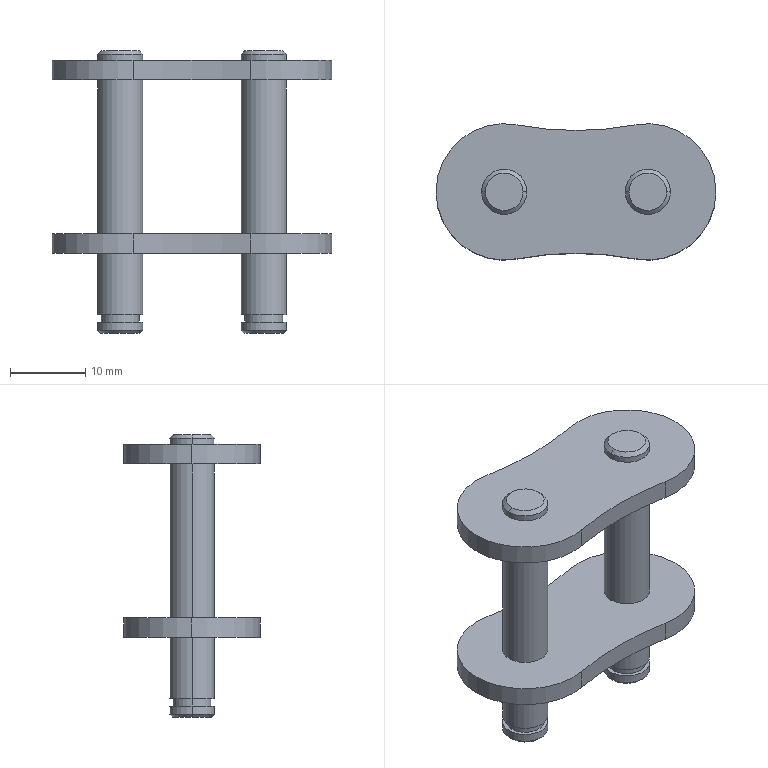Part | SolidWorks | features BaseBody 1 | 1 solid | 50 faces | box 37.13 x 18.08 x 37.5 mm | volume 4809 mm3 | cylinder 30 | plane 12 | cone 8 | commonest cylinder face diameters 6 x16 18.08 x6 5 x4 83.18 x4
STEP:
#1=CARTESIAN_POINT('',(-7.824,-8.879,2.59));
#2=VERTEX_POINT('',#1);
#3=CARTESIAN_POINT('',(-18.565,0.,2.59));
#4=VERTEX_POINT('',#3);
#5=CARTESIAN_POINT('',(-9.525,0.,2.59));
#6=DIRECTION('',(0.,0.,-1.));
#7=DIRECTION('',(-1.,0.,0.));
#8=AXIS2_PLACEMENT_3D('',#5,#6,#7);
#9=CIRCLE('',#8,9.04);
#10=EDGE_CURVE('',#2,#4,#9,.T.);
#11=ORIENTED_EDGE('',*,*,#10,.T.);
#12=CARTESIAN_POINT('',(-18.565,0.,0.));
#13=VERTEX_POINT('',#12);
#14=CARTESIAN_POINT('',(-18.565,0.,2.59));
#15=DIRECTION('',(0.,0.,-1.));
#16=VECTOR('',#15,1000.);
#17=LINE('',#14,#16);
#18=EDGE_CURVE('',#4,#13,#17,.T.);
#19=ORIENTED_EDGE('',*,*,#18,.T.);
#20=CARTESIAN_POINT('',(-7.824,-8.879,0.));
#21=VERTEX_POINT('',#20);
#22=CARTESIAN_POINT('',(-9.525,0.,0.));
#23=DIRECTION('',(0.,0.,-1.));
#24=DIRECTION('',(-1.,0.,0.));
#25=AXIS2_PLACEMENT_3D('',#22,#23,#24);
#26=CIRCLE('',#25,9.04);
#27=EDGE_CURVE('',#21,#13,#26,.T.);
#28=ORIENTED_EDGE('',*,*,#27,.F.);
#29=CARTESIAN_POINT('',(-7.824,-8.879,2.59));
#30=DIRECTION('',(0.,0.,1.));
#31=VECTOR('',#30,1000.);
#32=LINE('',#29,#31);
#33=EDGE_CURVE('',#21,#2,#32,.T.);
#34=ORIENTED_EDGE('',*,*,#33,.T.);
#35=EDGE_LOOP('',(#11,#19,#28,#34));
#36=FACE_OUTER_BOUND('',#35,.T.);
#37=CARTESIAN_POINT('',(-9.525,0.,2.59));
#38=DIRECTION('',(0.,0.,-1.));
#39=DIRECTION('',(-1.,0.,0.));
#40=AXIS2_PLACEMENT_3D('',#37,#38,#39);
#41=CYLINDRICAL_SURFACE('',#40,9.04);
#42=ADVANCED_FACE('',(#36),#41,.T.);
#43=CARTESIAN_POINT('',(12.525,0.,-20.41));
#44=VERTEX_POINT('',#43);
#45=CARTESIAN_POINT('',(6.525,0.,-20.41));
#46=VERTEX_POINT('',#45);
#47=CARTESIAN_POINT('',(9.525,0.,-20.41));
#48=DIRECTION('',(0.,0.,1.));
#49=DIRECTION('',(1.,0.,0.));
#50=AXIS2_PLACEMENT_3D('',#47,#48,#49);
#51=CIRCLE('',#50,3.);
#52=EDGE_CURVE('',#44,#46,#51,.T.);
#53=ORIENTED_EDGE('',*,*,#52,.T.);
#54=CARTESIAN_POINT('',(6.525,0.,0.));
#55=VERTEX_POINT('',#54);
#56=CARTESIAN_POINT('',(6.525,0.,3.89));
#57=DIRECTION('',(0.,0.,1.));
#58=VECTOR('',#57,1000.);
#59=LINE('',#56,#58);
#60=EDGE_CURVE('',#46,#55,#59,.T.);
#61=ORIENTED_EDGE('',*,*,#60,.T.);
#62=CARTESIAN_POINT('',(12.525,0.,0.));
#63=VERTEX_POINT('',#62);
#64=CARTESIAN_POINT('',(9.525,0.,0.));
#65=DIRECTION('',(0.,0.,1.));
#66=DIRECTION('',(1.,0.,0.));
#67=AXIS2_PLACEMENT_3D('',#64,#65,#66);
#68=CIRCLE('',#67,3.);
#69=EDGE_CURVE('',#63,#55,#68,.T.);
#70=ORIENTED_EDGE('',*,*,#69,.F.);
#71=CARTESIAN_POINT('',(12.525,0.,3.89));
#72=DIRECTION('',(0.,0.,1.));
#73=VECTOR('',#72,1000.);
#74=LINE('',#71,#73);
#75=EDGE_CURVE('',#44,#63,#74,.T.);
#76=ORIENTED_EDGE('',*,*,#75,.F.);
#77=EDGE_LOOP('',(#53,#61,#70,#76));
#78=FACE_OUTER_BOUND('',#77,.T.);
#79=CARTESIAN_POINT('',(9.525,0.,3.89));
#80=DIRECTION('',(0.,0.,1.));
#81=DIRECTION('',(1.,0.,0.));
#82=AXIS2_PLACEMENT_3D('',#79,#80,#81);
#83=CYLINDRICAL_SURFACE('',#82,3.);
#84=ADVANCED_FACE('',(#78),#83,.T.);
#85=CARTESIAN_POINT('',(-6.525,0.,-20.41));
#86=VERTEX_POINT('',#85);
#87=CARTESIAN_POINT('',(-12.525,0.,-20.41));
#88=VERTEX_POINT('',#87);
#89=CARTESIAN_POINT('',(-9.525,0.,-20.41));
#90=DIRECTION('',(0.,0.,1.));
#91=DIRECTION('',(1.,0.,0.));
#92=AXIS2_PLACEMENT_3D('',#89,#90,#91);
#93=CIRCLE('',#92,3.);
#94=EDGE_CURVE('',#86,#88,#93,.T.);
#95=ORIENTED_EDGE('',*,*,#94,.T.);
#96=CARTESIAN_POINT('',(-12.525,0.,0.));
#97=VERTEX_POINT('',#96);
#98=CARTESIAN_POINT('',(-12.525,0.,3.89));
#99=DIRECTION('',(0.,0.,1.));
#100=VECTOR('',#99,1000.);
#101=LINE('',#98,#100);
#102=EDGE_CURVE('',#88,#97,#101,.T.);
#103=ORIENTED_EDGE('',*,*,#102,.T.);
#104=CARTESIAN_POINT('',(-6.525,0.,0.));
#105=VERTEX_POINT('',#104);
#106=CARTESIAN_POINT('',(-9.525,0.,0.));
#107=DIRECTION('',(0.,0.,1.));
#108=DIRECTION('',(1.,0.,0.));
#109=AXIS2_PLACEMENT_3D('',#106,#107,#108);
#110=CIRCLE('',#109,3.);
#111=EDGE_CURVE('',#105,#97,#110,.T.);
#112=ORIENTED_EDGE('',*,*,#111,.F.);
#113=CARTESIAN_POINT('',(-6.525,0.,3.89));
#114=DIRECTION('',(0.,0.,1.));
#115=VECTOR('',#114,1000.);
#116=LINE('',#113,#115);
#117=EDGE_CURVE('',#86,#105,#116,.T.);
#118=ORIENTED_EDGE('',*,*,#117,.F.);
#119=EDGE_LOOP('',(#95,#103,#112,#118));
#120=FACE_OUTER_BOUND('',#119,.T.);
#121=CARTESIAN_POINT('',(-9.525,0.,3.89));
#122=DIRECTION('',(0.,0.,1.));
#123=DIRECTION('',(1.,0.,0.));
#124=AXIS2_PLACEMENT_3D('',#121,#122,#123);
#125=CYLINDRICAL_SURFACE('',#124,3.);
#126=ADVANCED_FACE('',(#120),#125,.T.);
#127=CARTESIAN_POINT('',(12.525,0.,2.59));
#128=VERTEX_POINT('',#127);
#129=CARTESIAN_POINT('',(6.525,0.,2.59));
#130=VERTEX_POINT('',#129);
#131=CARTESIAN_POINT('',(9.525,0.,2.59));
#132=DIRECTION('',(0.,0.,1.));
#133=DIRECTION('',(1.,0.,0.));
#134=AXIS2_PLACEMENT_3D('',#131,#132,#133);
#135=CIRCLE('',#134,3.);
#136=EDGE_CURVE('',#128,#130,#135,.T.);
#137=ORIENTED_EDGE('',*,*,#136,.T.);
#138=CARTESIAN_POINT('',(6.525,0.,3.39));
#139=VERTEX_POINT('',#138);
#140=CARTESIAN_POINT('',(6.525,0.,3.89));
#141=DIRECTION('',(0.,0.,1.));
#142=VECTOR('',#141,1000.);
#143=LINE('',#140,#142);
#144=EDGE_CURVE('',#130,#139,#143,.T.);
#145=ORIENTED_EDGE('',*,*,#144,.T.);
#146=CARTESIAN_POINT('',(12.525,0.,3.39));
#147=VERTEX_POINT('',#146);
#148=CARTESIAN_POINT('',(9.525,0.,3.39));
#149=DIRECTION('',(0.,0.,-1.));
#150=DIRECTION('',(1.,0.,0.));
#151=AXIS2_PLACEMENT_3D('',#148,#149,#150);
#152=CIRCLE('',#151,3.);
#153=EDGE_CURVE('',#139,#147,#152,.T.);
#154=ORIENTED_EDGE('',*,*,#153,.T.);
#155=CARTESIAN_POINT('',(12.525,0.,3.89));
#156=DIRECTION('',(0.,0.,1.));
#157=VECTOR('',#156,1000.);
#158=LINE('',#155,#157);
#159=EDGE_CURVE('',#128,#147,#158,.T.);
#160=ORIENTED_EDGE('',*,*,#159,.F.);
#161=EDGE_LOOP('',(#137,#145,#154,#160));
#162=FACE_OUTER_BOUND('',#161,.T.);
#163=CARTESIAN_POINT('',(9.525,0.,3.89));
#164=DIRECTION('',(0.,0.,1.));
#165=DIRECTION('',(1.,0.,0.));
#166=AXIS2_PLACEMENT_3D('',#163,#164,#165);
#167=CYLINDRICAL_SURFACE('',#166,3.);
#168=ADVANCED_FACE('',(#162),#167,.T.);
#169=CARTESIAN_POINT('',(-6.525,0.,2.59));
#170=VERTEX_POINT('',#169);
#171=CARTESIAN_POINT('',(-12.525,0.,2.59));
#172=VERTEX_POINT('',#171);
#173=CARTESIAN_POINT('',(-9.525,0.,2.59));
#174=DIRECTION('',(0.,0.,1.));
#175=DIRECTION('',(1.,0.,0.));
#176=AXIS2_PLACEMENT_3D('',#173,#174,#175);
#177=CIRCLE('',#176,3.);
#178=EDGE_CURVE('',#170,#172,#177,.T.);
#179=ORIENTED_EDGE('',*,*,#178,.T.);
#180=CARTESIAN_POINT('',(-12.525,0.,3.39));
#181=VERTEX_POINT('',#180);
#182=CARTESIAN_POINT('',(-12.525,0.,3.89));
#183=DIRECTION('',(0.,0.,1.));
#184=VECTOR('',#183,1000.);
#185=LINE('',#182,#184);
#186=EDGE_CURVE('',#172,#181,#185,.T.);
#187=ORIENTED_EDGE('',*,*,#186,.T.);
#188=CARTESIAN_POINT('',(-6.525,0.,3.39));
#189=VERTEX_POINT('',#188);
#190=CARTESIAN_POINT('',(-9.525,0.,3.39));
#191=DIRECTION('',(0.,0.,-1.));
#192=DIRECTION('',(1.,0.,0.));
#193=AXIS2_PLACEMENT_3D('',#190,#191,#192);
#194=CIRCLE('',#193,3.);
#195=EDGE_CURVE('',#181,#189,#194,.T.);
#196=ORIENTED_EDGE('',*,*,#195,.T.);
#197=CARTESIAN_POINT('',(-6.525,0.,3.89));
#198=DIRECTION('',(0.,0.,1.));
#199=VECTOR('',#198,1000.);
#200=LINE('',#197,#199);
#201=EDGE_CURVE('',#170,#189,#200,.T.);
#202=ORIENTED_EDGE('',*,*,#201,.F.);
#203=EDGE_LOOP('',(#179,#187,#196,#202));
#204=FACE_OUTER_BOUND('',#203,.T.);
#205=CARTESIAN_POINT('',(-9.525,0.,3.89));
#206=DIRECTION('',(0.,0.,1.));
#207=DIRECTION('',(1.,0.,0.));
#208=AXIS2_PLACEMENT_3D('',#205,#206,#207);
#209=CYLINDRICAL_SURFACE('',#208,3.);
#210=ADVANCED_FACE('',(#204),#209,.T.);
#211=CARTESIAN_POINT('',(-7.824,-8.879,-20.41));
#212=VERTEX_POINT('',#211);
#213=CARTESIAN_POINT('',(-18.565,0.,-20.41));
#214=VERTEX_POINT('',#213);
#215=CARTESIAN_POINT('',(-9.525,0.,-20.41));
#216=DIRECTION('',(0.,0.,-1.));
#217=DIRECTION('',(-1.,0.,0.));
#218=AXIS2_PLACEMENT_3D('',#215,#216,#217);
#219=CIRCLE('',#218,9.04);
#220=EDGE_CURVE('',#212,#214,#219,.T.);
#221=ORIENTED_EDGE('',*,*,#220,.T.);
#222=CARTESIAN_POINT('',(-18.565,0.,-23.));
#223=VERTEX_POINT('',#222);
#224=CARTESIAN_POINT('',(-18.565,0.,-20.41));
#225=DIRECTION('',(0.,0.,-1.));
#226=VECTOR('',#225,1000.);
#227=LINE('',#224,#226);
#228=EDGE_CURVE('',#214,#223,#227,.T.);
#229=ORIENTED_EDGE('',*,*,#228,.T.);
#230=CARTESIAN_POINT('',(-7.824,-8.879,-23.));
#231=VERTEX_POINT('',#230);
#232=CARTESIAN_POINT('',(-9.525,0.,-23.));
#233=DIRECTION('',(0.,0.,1.));
#234=DIRECTION('',(-1.,0.,0.));
#235=AXIS2_PLACEMENT_3D('',#232,#233,#234);
#236=CIRCLE('',#235,9.04);
#237=EDGE_CURVE('',#223,#231,#236,.T.);
#238=ORIENTED_EDGE('',*,*,#237,.T.);
#239=CARTESIAN_POINT('',(-7.824,-8.879,-20.41));
#240=DIRECTION('',(0.,0.,1.));
#241=VECTOR('',#240,1000.);
#242=LINE('',#239,#241);
#243=EDGE_CURVE('',#231,#212,#242,.T.);
#244=ORIENTED_EDGE('',*,*,#243,.T.);
#245=EDGE_LOOP('',(#221,#229,#238,#244));
#246=FACE_OUTER_BOUND('',#245,.T.);
#247=CARTESIAN_POINT('',(-9.525,0.,-20.41));
#248=DIRECTION('',(0.,0.,-1.));
#249=DIRECTION('',(-1.,0.,0.));
#250=AXIS2_PLACEMENT_3D('',#247,#248,#249);
#251=CYLINDRICAL_SURFACE('',#250,9.04);
#252=ADVANCED_FACE('',(#246),#251,.T.);
#253=CARTESIAN_POINT('',(7.025,0.,3.89));
#254=VERTEX_POINT('',#253);
#255=CARTESIAN_POINT('',(12.025,0.,3.89));
#256=VERTEX_POINT('',#255);
#257=CARTESIAN_POINT('',(9.525,0.,3.89));
#258=DIRECTION('',(0.,0.,-1.));
#259=DIRECTION('',(-1.,0.,0.));
#260=AXIS2_PLACEMENT_3D('',#257,#258,#259);
#261=CIRCLE('',#260,2.5);
#262=EDGE_CURVE('',#254,#256,#261,.T.);
#263=ORIENTED_EDGE('',*,*,#262,.T.);
#264=CARTESIAN_POINT('',(12.525,0.,3.39));
#265=DIRECTION('',(0.7071,0.,-0.7071));
#266=VECTOR('',#265,1000.);
#267=LINE('',#264,#266);
#268=EDGE_CURVE('',#256,#147,#267,.T.);
#269=ORIENTED_EDGE('',*,*,#268,.T.);
#270=ORIENTED_EDGE('',*,*,#153,.F.);
#271=CARTESIAN_POINT('',(6.525,0.,3.39));
#272=DIRECTION('',(-0.7071,0.,-0.7071));
#273=VECTOR('',#272,1000.);
#274=LINE('',#271,#273);
#275=EDGE_CURVE('',#254,#139,#274,.T.);
#276=ORIENTED_EDGE('',*,*,#275,.F.);
#277=EDGE_LOOP('',(#263,#269,#270,#276));
#278=FACE_OUTER_BOUND('',#277,.T.);
#279=CARTESIAN_POINT('',(9.525,0.,3.39));
#280=DIRECTION('',(0.,0.,-1.));
#281=DIRECTION('',(-1.,0.,0.));
#282=AXIS2_PLACEMENT_3D('',#279,#280,#281);
#283=CONICAL_SURFACE('',#282,3.,0.7854);
#284=ADVANCED_FACE('',(#278),#283,.T.);
#285=CARTESIAN_POINT('',(-12.025,0.,3.89));
#286=VERTEX_POINT('',#285);
#287=CARTESIAN_POINT('',(-7.025,0.,3.89));
#288=VERTEX_POINT('',#287);
#289=CARTESIAN_POINT('',(-9.525,0.,3.89));
#290=DIRECTION('',(0.,0.,-1.));
#291=DIRECTION('',(-1.,0.,0.));
#292=AXIS2_PLACEMENT_3D('',#289,#290,#291);
#293=CIRCLE('',#292,2.5);
#294=EDGE_CURVE('',#286,#288,#293,.T.);
#295=ORIENTED_EDGE('',*,*,#294,.T.);
#296=CARTESIAN_POINT('',(-6.525,0.,3.39));
#297=DIRECTION('',(0.7071,0.,-0.7071));
#298=VECTOR('',#297,1000.);
#299=LINE('',#296,#298);
#300=EDGE_CURVE('',#288,#189,#299,.T.);
#301=ORIENTED_EDGE('',*,*,#300,.T.);
#302=ORIENTED_EDGE('',*,*,#195,.F.);
#303=CARTESIAN_POINT('',(-12.525,0.,3.39));
#304=DIRECTION('',(-0.7071,0.,-0.7071));
#305=VECTOR('',#304,1000.);
#306=LINE('',#303,#305);
#307=EDGE_CURVE('',#286,#181,#306,.T.);
#308=ORIENTED_EDGE('',*,*,#307,.F.);
#309=EDGE_LOOP('',(#295,#301,#302,#308));
#310=FACE_OUTER_BOUND('',#309,.T.);
#311=CARTESIAN_POINT('',(-9.525,0.,3.39));
#312=DIRECTION('',(0.,0.,-1.));
#313=DIRECTION('',(-1.,0.,0.));
#314=AXIS2_PLACEMENT_3D('',#311,#312,#313);
#315=CONICAL_SURFACE('',#314,3.,0.7854);
#316=ADVANCED_FACE('',(#310),#315,.T.);
#317=CARTESIAN_POINT('',(-6.525,0.,-31.11));
#318=VERTEX_POINT('',#317);
#319=CARTESIAN_POINT('',(-12.525,0.,-31.11));
#320=VERTEX_POINT('',#319);
#321=CARTESIAN_POINT('',(-9.525,0.,-31.11));
#322=DIRECTION('',(0.,0.,1.));
#323=DIRECTION('',(1.,0.,0.));
#324=AXIS2_PLACEMENT_3D('',#321,#322,#323);
#325=CIRCLE('',#324,3.);
#326=EDGE_CURVE('',#318,#320,#325,.T.);
#327=ORIENTED_EDGE('',*,*,#326,.T.);
#328=CARTESIAN_POINT('',(-12.525,0.,-23.));
#329=VERTEX_POINT('',#328);
#330=CARTESIAN_POINT('',(-12.525,0.,3.89));
#331=DIRECTION('',(0.,0.,1.));
#332=VECTOR('',#331,1000.);
#333=LINE('',#330,#332);
#334=EDGE_CURVE('',#320,#329,#333,.T.);
#335=ORIENTED_EDGE('',*,*,#334,.T.);
#336=CARTESIAN_POINT('',(-6.525,0.,-23.));
#337=VERTEX_POINT('',#336);
#338=CARTESIAN_POINT('',(-9.525,0.,-23.));
#339=DIRECTION('',(0.,0.,1.));
#340=DIRECTION('',(1.,0.,0.));
#341=AXIS2_PLACEMENT_3D('',#338,#339,#340);
#342=CIRCLE('',#341,3.);
#343=EDGE_CURVE('',#337,#329,#342,.T.);
#344=ORIENTED_EDGE('',*,*,#343,.F.);
#345=CARTESIAN_POINT('',(-6.525,0.,3.89));
#346=DIRECTION('',(0.,0.,1.));
#347=VECTOR('',#346,1000.);
#348=LINE('',#345,#347);
#349=EDGE_CURVE('',#318,#337,#348,.T.);
#350=ORIENTED_EDGE('',*,*,#349,.F.);
#351=EDGE_LOOP('',(#327,#335,#344,#350));
#352=FACE_OUTER_BOUND('',#351,.T.);
#353=CARTESIAN_POINT('',(-9.525,0.,3.89));
#354=DIRECTION('',(0.,0.,1.));
#355=DIRECTION('',(1.,0.,0.));
#356=AXIS2_PLACEMENT_3D('',#353,#354,#355);
#357=CYLINDRICAL_SURFACE('',#356,3.);
#358=ADVANCED_FACE('',(#352),#357,.T.);
#359=CARTESIAN_POINT('',(12.525,0.,-31.11));
#360=VERTEX_POINT('',#359);
#361=CARTESIAN_POINT('',(6.525,0.,-31.11));
#362=VERTEX_POINT('',#361);
#363=CARTESIAN_POINT('',(9.525,0.,-31.11));
#364=DIRECTION('',(0.,0.,1.));
#365=DIRECTION('',(1.,0.,0.));
#366=AXIS2_PLACEMENT_3D('',#363,#364,#365);
#367=CIRCLE('',#366,3.);
#368=EDGE_CURVE('',#360,#362,#367,.T.);
#369=ORIENTED_EDGE('',*,*,#368,.T.);
#370=CARTESIAN_POINT('',(6.525,0.,-23.));
#371=VERTEX_POINT('',#370);
#372=CARTESIAN_POINT('',(6.525,0.,3.89));
#373=DIRECTION('',(0.,0.,1.));
#374=VECTOR('',#373,1000.);
#375=LINE('',#372,#374);
#376=EDGE_CURVE('',#362,#371,#375,.T.);
#377=ORIENTED_EDGE('',*,*,#376,.T.);
#378=CARTESIAN_POINT('',(12.525,0.,-23.));
#379=VERTEX_POINT('',#378);
#380=CARTESIAN_POINT('',(9.525,0.,-23.));
#381=DIRECTION('',(0.,0.,1.));
#382=DIRECTION('',(1.,0.,0.));
#383=AXIS2_PLACEMENT_3D('',#380,#381,#382);
#384=CIRCLE('',#383,3.);
#385=EDGE_CURVE('',#379,#371,#384,.T.);
#386=ORIENTED_EDGE('',*,*,#385,.F.);
#387=CARTESIAN_POINT('',(12.525,0.,3.89));
#388=DIRECTION('',(0.,0.,1.));
#389=VECTOR('',#388,1000.);
#390=LINE('',#387,#389);
#391=EDGE_CURVE('',#360,#379,#390,.T.);
#392=ORIENTED_EDGE('',*,*,#391,.F.);
#393=EDGE_LOOP('',(#369,#377,#386,#392));
#394=FACE_OUTER_BOUND('',#393,.T.);
#395=CARTESIAN_POINT('',(9.525,0.,3.89));
#396=DIRECTION('',(0.,0.,1.));
#397=DIRECTION('',(1.,0.,0.));
#398=AXIS2_PLACEMENT_3D('',#395,#396,#397);
#399=CYLINDRICAL_SURFACE('',#398,3.);
#400=ADVANCED_FACE('',(#394),#399,.T.);
#401=CARTESIAN_POINT('',(-7.025,0.,-32.11));
#402=VERTEX_POINT('',#401);
#403=CARTESIAN_POINT('',(-12.025,0.,-32.11));
#404=VERTEX_POINT('',#403);
#405=CARTESIAN_POINT('',(-9.525,0.,-32.11));
#406=DIRECTION('',(0.,0.,1.));
#407=DIRECTION('',(1.,0.,0.));
#408=AXIS2_PLACEMENT_3D('',#405,#406,#407);
#409=CIRCLE('',#408,2.5);
#410=EDGE_CURVE('',#402,#404,#409,.T.);
#411=ORIENTED_EDGE('',*,*,#410,.T.);
#412=CARTESIAN_POINT('',(-12.025,0.,-31.11));
#413=VERTEX_POINT('',#412);
#414=CARTESIAN_POINT('',(-12.025,0.,3.89));
#415=DIRECTION('',(0.,0.,1.));
#416=VECTOR('',#415,1000.);
#417=LINE('',#414,#416);
#418=EDGE_CURVE('',#404,#413,#417,.T.);
#419=ORIENTED_EDGE('',*,*,#418,.T.);
#420=CARTESIAN_POINT('',(-7.025,0.,-31.11));
#421=VERTEX_POINT('',#420);
#422=CARTESIAN_POINT('',(-9.525,0.,-31.11));
#423=DIRECTION('',(0.,0.,1.));
#424=DIRECTION('',(1.,0.,0.));
#425=AXIS2_PLACEMENT_3D('',#422,#423,#424);
#426=CIRCLE('',#425,2.5);
#427=EDGE_CURVE('',#421,#413,#426,.T.);
#428=ORIENTED_EDGE('',*,*,#427,.F.);
#429=CARTESIAN_POINT('',(-7.025,0.,3.89));
#430=DIRECTION('',(0.,0.,1.));
#431=VECTOR('',#430,1000.);
#432=LINE('',#429,#431);
#433=EDGE_CURVE('',#402,#421,#432,.T.);
#434=ORIENTED_EDGE('',*,*,#433,.F.);
#435=EDGE_LOOP('',(#411,#419,#428,#434));
#436=FACE_OUTER_BOUND('',#435,.T.);
#437=CARTESIAN_POINT('',(-9.525,0.,3.89));
#438=DIRECTION('',(0.,0.,1.));
#439=DIRECTION('',(1.,0.,0.));
#440=AXIS2_PLACEMENT_3D('',#437,#438,#439);
#441=CYLINDRICAL_SURFACE('',#440,2.5);
#442=ADVANCED_FACE('',(#436),#441,.T.);
#443=CARTESIAN_POINT('',(12.025,0.,-32.11));
#444=VERTEX_POINT('',#443);
#445=CARTESIAN_POINT('',(7.025,0.,-32.11));
#446=VERTEX_POINT('',#445);
#447=CARTESIAN_POINT('',(9.525,0.,-32.11));
#448=DIRECTION('',(0.,0.,1.));
#449=DIRECTION('',(1.,0.,0.));
#450=AXIS2_PLACEMENT_3D('',#447,#448,#449);
#451=CIRCLE('',#450,2.5);
#452=EDGE_CURVE('',#444,#446,#451,.T.);
#453=ORIENTED_EDGE('',*,*,#452,.T.);
#454=CARTESIAN_POINT('',(7.025,0.,-31.11));
#455=VERTEX_POINT('',#454);
#456=CARTESIAN_POINT('',(7.025,0.,3.89));
#457=DIRECTION('',(0.,0.,1.));
#458=VECTOR('',#457,1000.);
#459=LINE('',#456,#458);
#460=EDGE_CURVE('',#446,#455,#459,.T.);
#461=ORIENTED_EDGE('',*,*,#460,.T.);
#462=CARTESIAN_POINT('',(12.025,0.,-31.11));
#463=VERTEX_POINT('',#462);
#464=CARTESIAN_POINT('',(9.525,0.,-31.11));
#465=DIRECTION('',(0.,0.,1.));
#466=DIRECTION('',(1.,0.,0.));
#467=AXIS2_PLACEMENT_3D('',#464,#465,#466);
#468=CIRCLE('',#467,2.5);
#469=EDGE_CURVE('',#463,#455,#468,.T.);
#470=ORIENTED_EDGE('',*,*,#469,.F.);
#471=CARTESIAN_POINT('',(12.025,0.,3.89));
#472=DIRECTION('',(0.,0.,1.));
#473=VECTOR('',#472,1000.);
#474=LINE('',#471,#473);
#475=EDGE_CURVE('',#444,#463,#474,.T.);
#476=ORIENTED_EDGE('',*,*,#475,.F.);
#477=EDGE_LOOP('',(#453,#461,#470,#476));
#478=FACE_OUTER_BOUND('',#477,.T.);
#479=CARTESIAN_POINT('',(9.525,0.,3.89));
#480=DIRECTION('',(0.,0.,1.));
#481=DIRECTION('',(1.,0.,0.));
#482=AXIS2_PLACEMENT_3D('',#479,#480,#481);
#483=CYLINDRICAL_SURFACE('',#482,2.5);
#484=ADVANCED_FACE('',(#478),#483,.T.);
#485=CARTESIAN_POINT('',(-6.525,0.,-33.21));
#486=VERTEX_POINT('',#485);
#487=CARTESIAN_POINT('',(-12.525,0.,-33.21));
#488=VERTEX_POINT('',#487);
#489=CARTESIAN_POINT('',(-9.525,0.,-33.21));
#490=DIRECTION('',(0.,0.,1.));
#491=DIRECTION('',(1.,0.,0.));
#492=AXIS2_PLACEMENT_3D('',#489,#490,#491);
#493=CIRCLE('',#492,3.);
#494=EDGE_CURVE('',#486,#488,#493,.T.);
#495=ORIENTED_EDGE('',*,*,#494,.T.);
#496=CARTESIAN_POINT('',(-12.525,0.,-32.11));
#497=VERTEX_POINT('',#496);
#498=CARTESIAN_POINT('',(-12.525,0.,3.89));
#499=DIRECTION('',(0.,0.,1.));
#500=VECTOR('',#499,1000.);
#501=LINE('',#498,#500);
#502=EDGE_CURVE('',#488,#497,#501,.T.);
#503=ORIENTED_EDGE('',*,*,#502,.T.);
#504=CARTESIAN_POINT('',(-6.525,0.,-32.11));
#505=VERTEX_POINT('',#504);
#506=CARTESIAN_POINT('',(-9.525,0.,-32.11));
#507=DIRECTION('',(0.,0.,1.));
#508=DIRECTION('',(1.,0.,0.));
#509=AXIS2_PLACEMENT_3D('',#506,#507,#508);
#510=CIRCLE('',#509,3.);
#511=EDGE_CURVE('',#505,#497,#510,.T.);
#512=ORIENTED_EDGE('',*,*,#511,.F.);
#513=CARTESIAN_POINT('',(-6.525,0.,3.89));
#514=DIRECTION('',(0.,0.,1.));
#515=VECTOR('',#514,1000.);
#516=LINE('',#513,#515);
#517=EDGE_CURVE('',#486,#505,#516,.T.);
#518=ORIENTED_EDGE('',*,*,#517,.F.);
#519=EDGE_LOOP('',(#495,#503,#512,#518));
#520=FACE_OUTER_BOUND('',#519,.T.);
#521=CARTESIAN_POINT('',(-9.525,0.,3.89));
#522=DIRECTION('',(0.,0.,1.));
#523=DIRECTION('',(1.,0.,0.));
#524=AXIS2_PLACEMENT_3D('',#521,#522,#523);
#525=CYLINDRICAL_SURFACE('',#524,3.);
#526=ADVANCED_FACE('',(#520),#525,.T.);
#527=CARTESIAN_POINT('',(12.525,0.,-33.21));
#528=VERTEX_POINT('',#527);
#529=CARTESIAN_POINT('',(6.525,0.,-33.21));
#530=VERTEX_POINT('',#529);
#531=CARTESIAN_POINT('',(9.525,0.,-33.21));
#532=DIRECTION('',(0.,0.,1.));
#533=DIRECTION('',(1.,0.,0.));
#534=AXIS2_PLACEMENT_3D('',#531,#532,#533);
#535=CIRCLE('',#534,3.);
#536=EDGE_CURVE('',#528,#530,#535,.T.);
#537=ORIENTED_EDGE('',*,*,#536,.T.);
#538=CARTESIAN_POINT('',(6.525,0.,-32.11));
#539=VERTEX_POINT('',#538);
#540=CARTESIAN_POINT('',(6.525,0.,3.89));
#541=DIRECTION('',(0.,0.,1.));
#542=VECTOR('',#541,1000.);
#543=LINE('',#540,#542);
#544=EDGE_CURVE('',#530,#539,#543,.T.);
#545=ORIENTED_EDGE('',*,*,#544,.T.);
#546=CARTESIAN_POINT('',(12.525,0.,-32.11));
#547=VERTEX_POINT('',#546);
#548=CARTESIAN_POINT('',(9.525,0.,-32.11));
#549=DIRECTION('',(0.,0.,1.));
#550=DIRECTION('',(1.,0.,0.));
#551=AXIS2_PLACEMENT_3D('',#548,#549,#550);
#552=CIRCLE('',#551,3.);
#553=EDGE_CURVE('',#547,#539,#552,.T.);
#554=ORIENTED_EDGE('',*,*,#553,.F.);
#555=CARTESIAN_POINT('',(12.525,0.,3.89));
#556=DIRECTION('',(0.,0.,1.));
#557=VECTOR('',#556,1000.);
#558=LINE('',#555,#557);
#559=EDGE_CURVE('',#528,#547,#558,.T.);
#560=ORIENTED_EDGE('',*,*,#559,.F.);
#561=EDGE_LOOP('',(#537,#545,#554,#560));
#562=FACE_OUTER_BOUND('',#561,.T.);
#563=CARTESIAN_POINT('',(9.525,0.,3.89));
#564=DIRECTION('',(0.,0.,1.));
#565=DIRECTION('',(1.,0.,0.));
#566=AXIS2_PLACEMENT_3D('',#563,#564,#565);
#567=CYLINDRICAL_SURFACE('',#566,3.);
#568=ADVANCED_FACE('',(#562),#567,.T.);
#569=CARTESIAN_POINT('',(-6.925,0.,-33.61));
#570=VERTEX_POINT('',#569);
#571=CARTESIAN_POINT('',(-12.125,0.,-33.61));
#572=VERTEX_POINT('',#571);
#573=CARTESIAN_POINT('',(-9.525,0.,-33.61));
#574=DIRECTION('',(0.,0.,1.));
#575=DIRECTION('',(1.,0.,0.));
#576=AXIS2_PLACEMENT_3D('',#573,#574,#575);
#577=CIRCLE('',#576,2.6);
#578=EDGE_CURVE('',#570,#572,#577,.T.);
#579=ORIENTED_EDGE('',*,*,#578,.T.);
#580=CARTESIAN_POINT('',(-12.525,0.,-33.21));
#581=DIRECTION('',(-0.7071,0.,0.7071));
#582=VECTOR('',#581,1000.);
#583=LINE('',#580,#582);
#584=EDGE_CURVE('',#572,#488,#583,.T.);
#585=ORIENTED_EDGE('',*,*,#584,.T.);
#586=ORIENTED_EDGE('',*,*,#494,.F.);
#587=CARTESIAN_POINT('',(-6.525,0.,-33.21));
#588=DIRECTION('',(0.7071,0.,0.7071));
#589=VECTOR('',#588,1000.);
#590=LINE('',#587,#589);
#591=EDGE_CURVE('',#570,#486,#590,.T.);
#592=ORIENTED_EDGE('',*,*,#591,.F.);
#593=EDGE_LOOP('',(#579,#585,#586,#592));
#594=FACE_OUTER_BOUND('',#593,.T.);
#595=CARTESIAN_POINT('',(-9.525,0.,-33.21));
#596=DIRECTION('',(0.,0.,1.));
#597=DIRECTION('',(1.,0.,0.));
#598=AXIS2_PLACEMENT_3D('',#595,#596,#597);
#599=CONICAL_SURFACE('',#598,3.,0.7854);
#600=ADVANCED_FACE('',(#594),#599,.T.);
#601=CARTESIAN_POINT('',(12.125,0.,-33.61));
#602=VERTEX_POINT('',#601);
#603=CARTESIAN_POINT('',(6.925,0.,-33.61));
#604=VERTEX_POINT('',#603);
#605=CARTESIAN_POINT('',(9.525,0.,-33.61));
#606=DIRECTION('',(0.,0.,1.));
#607=DIRECTION('',(1.,0.,0.));
#608=AXIS2_PLACEMENT_3D('',#605,#606,#607);
#609=CIRCLE('',#608,2.6);
#610=EDGE_CURVE('',#602,#604,#609,.T.);
#611=ORIENTED_EDGE('',*,*,#610,.T.);
#612=CARTESIAN_POINT('',(6.525,0.,-33.21));
#613=DIRECTION('',(-0.7071,0.,0.7071));
#614=VECTOR('',#613,1000.);
#615=LINE('',#612,#614);
#616=EDGE_CURVE('',#604,#530,#615,.T.);
#617=ORIENTED_EDGE('',*,*,#616,.T.);
#618=ORIENTED_EDGE('',*,*,#536,.F.);
#619=CARTESIAN_POINT('',(12.525,0.,-33.21));
#620=DIRECTION('',(0.7071,0.,0.7071));
#621=VECTOR('',#620,1000.);
#622=LINE('',#619,#621);
#623=EDGE_CURVE('',#602,#528,#622,.T.);
#624=ORIENTED_EDGE('',*,*,#623,.F.);
#625=EDGE_LOOP('',(#611,#617,#618,#624));
#626=FACE_OUTER_BOUND('',#625,.T.);
#627=CARTESIAN_POINT('',(9.525,0.,-33.21));
#628=DIRECTION('',(0.,0.,1.));
#629=DIRECTION('',(1.,0.,0.));
#630=AXIS2_PLACEMENT_3D('',#627,#628,#629);
#631=CONICAL_SURFACE('',#630,3.,0.7854);
#632=ADVANCED_FACE('',(#626),#631,.T.);
#633=CARTESIAN_POINT('',(-7.824,8.879,0.));
#634=VERTEX_POINT('',#633);
#635=CARTESIAN_POINT('',(7.824,8.879,0.));
#636=VERTEX_POINT('',#635);
#637=CARTESIAN_POINT('',(0.,49.726,0.));
#638=DIRECTION('',(0.,0.,1.));
#639=DIRECTION('',(-1.,0.,0.));
#640=AXIS2_PLACEMENT_3D('',#637,#638,#639);
#641=CIRCLE('',#640,41.59);
#642=EDGE_CURVE('',#634,#636,#641,.T.);
#643=ORIENTED_EDGE('',*,*,#642,.T.);
#644=CARTESIAN_POINT('',(7.824,-8.879,0.));
#645=VERTEX_POINT('',#644);
#646=CARTESIAN_POINT('',(9.525,0.,0.));
#647=DIRECTION('',(0.,0.,-1.));
#648=DIRECTION('',(-1.,0.,0.));
#649=AXIS2_PLACEMENT_3D('',#646,#647,#648);
#650=CIRCLE('',#649,9.04);
#651=EDGE_CURVE('',#636,#645,#650,.T.);
#652=ORIENTED_EDGE('',*,*,#651,.T.);
#653=CARTESIAN_POINT('',(0.,-49.726,0.));
#654=DIRECTION('',(0.,0.,1.));
#655=DIRECTION('',(-1.,0.,0.));
#656=AXIS2_PLACEMENT_3D('',#653,#654,#655);
#657=CIRCLE('',#656,41.59);
#658=EDGE_CURVE('',#645,#21,#657,.T.);
#659=ORIENTED_EDGE('',*,*,#658,.T.);
#660=ORIENTED_EDGE('',*,*,#27,.T.);
#661=CARTESIAN_POINT('',(-9.525,0.,0.));
#662=DIRECTION('',(0.,0.,-1.));
#663=DIRECTION('',(-1.,0.,0.));
#664=AXIS2_PLACEMENT_3D('',#661,#662,#663);
#665=CIRCLE('',#664,9.04);
#666=EDGE_CURVE('',#13,#634,#665,.T.);
#667=ORIENTED_EDGE('',*,*,#666,.T.);
#668=EDGE_LOOP('',(#643,#652,#659,#660,#667));
#669=FACE_OUTER_BOUND('',#668,.T.);
#670=ORIENTED_EDGE('',*,*,#69,.T.);
#671=CARTESIAN_POINT('',(9.525,0.,0.));
#672=DIRECTION('',(0.,0.,1.));
#673=DIRECTION('',(1.,0.,0.));
#674=AXIS2_PLACEMENT_3D('',#671,#672,#673);
#675=CIRCLE('',#674,3.);
#676=EDGE_CURVE('',#55,#63,#675,.T.);
#677=ORIENTED_EDGE('',*,*,#676,.T.);
#678=EDGE_LOOP('',(#670,#677));
#679=FACE_BOUND('',#678,.T.);
#680=ORIENTED_EDGE('',*,*,#111,.T.);
#681=CARTESIAN_POINT('',(-9.525,0.,0.));
#682=DIRECTION('',(0.,0.,1.));
#683=DIRECTION('',(1.,0.,0.));
#684=AXIS2_PLACEMENT_3D('',#681,#682,#683);
#685=CIRCLE('',#684,3.);
#686=EDGE_CURVE('',#97,#105,#685,.T.);
#687=ORIENTED_EDGE('',*,*,#686,.T.);
#688=EDGE_LOOP('',(#680,#687));
#689=FACE_BOUND('',#688,.T.);
#690=CARTESIAN_POINT('',(4.763,-24.863,0.));
#691=DIRECTION('',(0.,0.,-1.));
#692=DIRECTION('',(-1.,0.,0.));
#693=AXIS2_PLACEMENT_3D('',#690,#691,#692);
#694=PLANE('',#693);
#695=ADVANCED_FACE('',(#669,#679,#689),#694,.T.);
#696=CARTESIAN_POINT('',(7.824,8.879,2.59));
#697=VERTEX_POINT('',#696);
#698=CARTESIAN_POINT('',(7.824,-8.879,2.59));
#699=VERTEX_POINT('',#698);
#700=CARTESIAN_POINT('',(9.525,0.,2.59));
#701=DIRECTION('',(0.,0.,-1.));
#702=DIRECTION('',(-1.,0.,0.));
#703=AXIS2_PLACEMENT_3D('',#700,#701,#702);
#704=CIRCLE('',#703,9.04);
#705=EDGE_CURVE('',#697,#699,#704,.T.);
#706=ORIENTED_EDGE('',*,*,#705,.T.);
#707=CARTESIAN_POINT('',(7.824,-8.879,2.59));
#708=DIRECTION('',(0.,0.,-1.));
#709=VECTOR('',#708,1000.);
#710=LINE('',#707,#709);
#711=EDGE_CURVE('',#699,#645,#710,.T.);
#712=ORIENTED_EDGE('',*,*,#711,.T.);
#713=ORIENTED_EDGE('',*,*,#651,.F.);
#714=CARTESIAN_POINT('',(7.824,8.879,2.59));
#715=DIRECTION('',(0.,0.,1.));
#716=VECTOR('',#715,1000.);
#717=LINE('',#714,#716);
#718=EDGE_CURVE('',#636,#697,#717,.T.);
#719=ORIENTED_EDGE('',*,*,#718,.T.);
#720=EDGE_LOOP('',(#706,#712,#713,#719));
#721=FACE_OUTER_BOUND('',#720,.T.);
#722=CARTESIAN_POINT('',(9.525,0.,2.59));
#723=DIRECTION('',(0.,0.,-1.));
#724=DIRECTION('',(-1.,0.,0.));
#725=AXIS2_PLACEMENT_3D('',#722,#723,#724);
#726=CYLINDRICAL_SURFACE('',#725,9.04);
#727=ADVANCED_FACE('',(#721),#726,.T.);
#728=CARTESIAN_POINT('',(-7.824,8.879,2.59));
#729=VERTEX_POINT('',#728);
#730=CARTESIAN_POINT('',(-7.824,8.879,2.59));
#731=DIRECTION('',(0.,0.,-1.));
#732=VECTOR('',#731,1000.);
#733=LINE('',#730,#732);
#734=EDGE_CURVE('',#729,#634,#733,.T.);
#735=ORIENTED_EDGE('',*,*,#734,.F.);
#736=CARTESIAN_POINT('',(0.,49.726,2.59));
#737=DIRECTION('',(0.,0.,-1.));
#738=DIRECTION('',(-1.,0.,0.));
#739=AXIS2_PLACEMENT_3D('',#736,#737,#738);
#740=CIRCLE('',#739,41.59);
#741=EDGE_CURVE('',#697,#729,#740,.T.);
#742=ORIENTED_EDGE('',*,*,#741,.F.);
#743=ORIENTED_EDGE('',*,*,#718,.F.);
#744=ORIENTED_EDGE('',*,*,#642,.F.);
#745=EDGE_LOOP('',(#735,#742,#743,#744));
#746=FACE_OUTER_BOUND('',#745,.T.);
#747=CARTESIAN_POINT('',(0.,49.726,2.59));
#748=DIRECTION('',(0.,0.,-1.));
#749=DIRECTION('',(-1.,0.,0.));
#750=AXIS2_PLACEMENT_3D('',#747,#748,#749);
#751=CYLINDRICAL_SURFACE('',#750,41.59);
#752=ADVANCED_FACE('',(#746),#751,.F.);
#753=ORIENTED_EDGE('',*,*,#18,.F.);
#754=CARTESIAN_POINT('',(-9.525,0.,2.59));
#755=DIRECTION('',(0.,0.,-1.));
#756=DIRECTION('',(-1.,0.,0.));
#757=AXIS2_PLACEMENT_3D('',#754,#755,#756);
#758=CIRCLE('',#757,9.04);
#759=EDGE_CURVE('',#4,#729,#758,.T.);
#760=ORIENTED_EDGE('',*,*,#759,.T.);
#761=ORIENTED_EDGE('',*,*,#734,.T.);
#762=ORIENTED_EDGE('',*,*,#666,.F.);
#763=EDGE_LOOP('',(#753,#760,#761,#762));
#764=FACE_OUTER_BOUND('',#763,.T.);
#765=CARTESIAN_POINT('',(-9.525,0.,2.59));
#766=DIRECTION('',(0.,0.,-1.));
#767=DIRECTION('',(-1.,0.,0.));
#768=AXIS2_PLACEMENT_3D('',#765,#766,#767);
#769=CYLINDRICAL_SURFACE('',#768,9.04);
#770=ADVANCED_FACE('',(#764),#769,.T.);
#771=ORIENTED_EDGE('',*,*,#711,.F.);
#772=CARTESIAN_POINT('',(0.,-49.726,2.59));
#773=DIRECTION('',(0.,0.,-1.));
#774=DIRECTION('',(-1.,0.,0.));
#775=AXIS2_PLACEMENT_3D('',#772,#773,#774);
#776=CIRCLE('',#775,41.59);
#777=EDGE_CURVE('',#2,#699,#776,.T.);
#778=ORIENTED_EDGE('',*,*,#777,.F.);
#779=ORIENTED_EDGE('',*,*,#33,.F.);
#780=ORIENTED_EDGE('',*,*,#658,.F.);
#781=EDGE_LOOP('',(#771,#778,#779,#780));
#782=FACE_OUTER_BOUND('',#781,.T.);
#783=CARTESIAN_POINT('',(0.,-49.726,2.59));
#784=DIRECTION('',(0.,0.,-1.));
#785=DIRECTION('',(-1.,0.,0.));
#786=AXIS2_PLACEMENT_3D('',#783,#784,#785);
#787=CYLINDRICAL_SURFACE('',#786,41.59);
#788=ADVANCED_FACE('',(#782),#787,.F.);
#789=ORIENTED_EDGE('',*,*,#60,.F.);
#790=CARTESIAN_POINT('',(9.525,0.,-20.41));
#791=DIRECTION('',(0.,0.,1.));
#792=DIRECTION('',(1.,0.,0.));
#793=AXIS2_PLACEMENT_3D('',#790,#791,#792);
#794=CIRCLE('',#793,3.);
#795=EDGE_CURVE('',#46,#44,#794,.T.);
#796=ORIENTED_EDGE('',*,*,#795,.T.);
#797=ORIENTED_EDGE('',*,*,#75,.T.);
#798=ORIENTED_EDGE('',*,*,#676,.F.);
#799=EDGE_LOOP('',(#789,#796,#797,#798));
#800=FACE_OUTER_BOUND('',#799,.T.);
#801=CARTESIAN_POINT('',(9.525,0.,3.89));
#802=DIRECTION('',(0.,0.,1.));
#803=DIRECTION('',(1.,0.,0.));
#804=AXIS2_PLACEMENT_3D('',#801,#802,#803);
#805=CYLINDRICAL_SURFACE('',#804,3.);
#806=ADVANCED_FACE('',(#800),#805,.T.);
#807=ORIENTED_EDGE('',*,*,#102,.F.);
#808=CARTESIAN_POINT('',(-9.525,0.,-20.41));
#809=DIRECTION('',(0.,0.,1.));
#810=DIRECTION('',(1.,0.,0.));
#811=AXIS2_PLACEMENT_3D('',#808,#809,#810);
#812=CIRCLE('',#811,3.);
#813=EDGE_CURVE('',#88,#86,#812,.T.);
#814=ORIENTED_EDGE('',*,*,#813,.T.);
#815=ORIENTED_EDGE('',*,*,#117,.T.);
#816=ORIENTED_EDGE('',*,*,#686,.F.);
#817=EDGE_LOOP('',(#807,#814,#815,#816));
#818=FACE_OUTER_BOUND('',#817,.T.);
#819=CARTESIAN_POINT('',(-9.525,0.,3.89));
#820=DIRECTION('',(0.,0.,1.));
#821=DIRECTION('',(1.,0.,0.));
#822=AXIS2_PLACEMENT_3D('',#819,#820,#821);
#823=CYLINDRICAL_SURFACE('',#822,3.);
#824=ADVANCED_FACE('',(#818),#823,.T.);
#825=ORIENTED_EDGE('',*,*,#705,.F.);
#826=ORIENTED_EDGE('',*,*,#741,.T.);
#827=ORIENTED_EDGE('',*,*,#759,.F.);
#828=ORIENTED_EDGE('',*,*,#10,.F.);
#829=ORIENTED_EDGE('',*,*,#777,.T.);
#830=EDGE_LOOP('',(#825,#826,#827,#828,#829));
#831=FACE_OUTER_BOUND('',#830,.T.);
#832=ORIENTED_EDGE('',*,*,#136,.F.);
#833=CARTESIAN_POINT('',(9.525,0.,2.59));
#834=DIRECTION('',(0.,0.,1.));
#835=DIRECTION('',(1.,0.,0.));
#836=AXIS2_PLACEMENT_3D('',#833,#834,#835);
#837=CIRCLE('',#836,3.);
#838=EDGE_CURVE('',#130,#128,#837,.T.);
#839=ORIENTED_EDGE('',*,*,#838,.F.);
#840=EDGE_LOOP('',(#832,#839));
#841=FACE_BOUND('',#840,.T.);
#842=ORIENTED_EDGE('',*,*,#178,.F.);
#843=CARTESIAN_POINT('',(-9.525,0.,2.59));
#844=DIRECTION('',(0.,0.,1.));
#845=DIRECTION('',(1.,0.,0.));
#846=AXIS2_PLACEMENT_3D('',#843,#844,#845);
#847=CIRCLE('',#846,3.);
#848=EDGE_CURVE('',#172,#170,#847,.T.);
#849=ORIENTED_EDGE('',*,*,#848,.F.);
#850=EDGE_LOOP('',(#842,#849));
#851=FACE_BOUND('',#850,.T.);
#852=CARTESIAN_POINT('',(4.763,-24.863,2.59));
#853=DIRECTION('',(0.,0.,-1.));
#854=DIRECTION('',(-1.,0.,0.));
#855=AXIS2_PLACEMENT_3D('',#852,#853,#854);
#856=PLANE('',#855);
#857=ADVANCED_FACE('',(#831,#841,#851),#856,.F.);
#858=CARTESIAN_POINT('',(7.824,8.879,-20.41));
#859=VERTEX_POINT('',#858);
#860=CARTESIAN_POINT('',(7.824,-8.879,-20.41));
#861=VERTEX_POINT('',#860);
#862=CARTESIAN_POINT('',(9.525,0.,-20.41));
#863=DIRECTION('',(0.,0.,-1.));
#864=DIRECTION('',(-1.,0.,0.));
#865=AXIS2_PLACEMENT_3D('',#862,#863,#864);
#866=CIRCLE('',#865,9.04);
#867=EDGE_CURVE('',#859,#861,#866,.T.);
#868=ORIENTED_EDGE('',*,*,#867,.F.);
#869=CARTESIAN_POINT('',(-7.824,8.879,-20.41));
#870=VERTEX_POINT('',#869);
#871=CARTESIAN_POINT('',(0.,49.726,-20.41));
#872=DIRECTION('',(0.,0.,1.));
#873=DIRECTION('',(-1.,0.,0.));
#874=AXIS2_PLACEMENT_3D('',#871,#872,#873);
#875=CIRCLE('',#874,41.59);
#876=EDGE_CURVE('',#870,#859,#875,.T.);
#877=ORIENTED_EDGE('',*,*,#876,.F.);
#878=CARTESIAN_POINT('',(-9.525,0.,-20.41));
#879=DIRECTION('',(0.,0.,-1.));
#880=DIRECTION('',(-1.,0.,0.));
#881=AXIS2_PLACEMENT_3D('',#878,#879,#880);
#882=CIRCLE('',#881,9.04);
#883=EDGE_CURVE('',#214,#870,#882,.T.);
#884=ORIENTED_EDGE('',*,*,#883,.F.);
#885=ORIENTED_EDGE('',*,*,#220,.F.);
#886=CARTESIAN_POINT('',(0.,-49.726,-20.41));
#887=DIRECTION('',(0.,0.,1.));
#888=DIRECTION('',(-1.,0.,0.));
#889=AXIS2_PLACEMENT_3D('',#886,#887,#888);
#890=CIRCLE('',#889,41.59);
#891=EDGE_CURVE('',#861,#212,#890,.T.);
#892=ORIENTED_EDGE('',*,*,#891,.F.);
#893=EDGE_LOOP('',(#868,#877,#884,#885,#892));
#894=FACE_OUTER_BOUND('',#893,.T.);
#895=ORIENTED_EDGE('',*,*,#94,.F.);
#896=ORIENTED_EDGE('',*,*,#813,.F.);
#897=EDGE_LOOP('',(#895,#896));
#898=FACE_BOUND('',#897,.T.);
#899=ORIENTED_EDGE('',*,*,#52,.F.);
#900=ORIENTED_EDGE('',*,*,#795,.F.);
#901=EDGE_LOOP('',(#899,#900));
#902=FACE_BOUND('',#901,.T.);
#903=CARTESIAN_POINT('',(4.763,-24.863,-20.41));
#904=DIRECTION('',(0.,0.,-1.));
#905=DIRECTION('',(-1.,0.,0.));
#906=AXIS2_PLACEMENT_3D('',#903,#904,#905);
#907=PLANE('',#906);
#908=ADVANCED_FACE('',(#894,#898,#902),#907,.F.);
#909=ORIENTED_EDGE('',*,*,#144,.F.);
#910=ORIENTED_EDGE('',*,*,#838,.T.);
#911=ORIENTED_EDGE('',*,*,#159,.T.);
#912=CARTESIAN_POINT('',(9.525,0.,3.39));
#913=DIRECTION('',(0.,0.,-1.));
#914=DIRECTION('',(1.,0.,0.));
#915=AXIS2_PLACEMENT_3D('',#912,#913,#914);
#916=CIRCLE('',#915,3.);
#917=EDGE_CURVE('',#147,#139,#916,.T.);
#918=ORIENTED_EDGE('',*,*,#917,.T.);
#919=EDGE_LOOP('',(#909,#910,#911,#918));
#920=FACE_OUTER_BOUND('',#919,.T.);
#921=CARTESIAN_POINT('',(9.525,0.,3.89));
#922=DIRECTION('',(0.,0.,1.));
#923=DIRECTION('',(1.,0.,0.));
#924=AXIS2_PLACEMENT_3D('',#921,#922,#923);
#925=CYLINDRICAL_SURFACE('',#924,3.);
#926=ADVANCED_FACE('',(#920),#925,.T.);
#927=ORIENTED_EDGE('',*,*,#186,.F.);
#928=ORIENTED_EDGE('',*,*,#848,.T.);
#929=ORIENTED_EDGE('',*,*,#201,.T.);
#930=CARTESIAN_POINT('',(-9.525,0.,3.39));
#931=DIRECTION('',(0.,0.,-1.));
#932=DIRECTION('',(1.,0.,0.));
#933=AXIS2_PLACEMENT_3D('',#930,#931,#932);
#934=CIRCLE('',#933,3.);
#935=EDGE_CURVE('',#189,#181,#934,.T.);
#936=ORIENTED_EDGE('',*,*,#935,.T.);
#937=EDGE_LOOP('',(#927,#928,#929,#936));
#938=FACE_OUTER_BOUND('',#937,.T.);
#939=CARTESIAN_POINT('',(-9.525,0.,3.89));
#940=DIRECTION('',(0.,0.,1.));
#941=DIRECTION('',(1.,0.,0.));
#942=AXIS2_PLACEMENT_3D('',#939,#940,#941);
#943=CYLINDRICAL_SURFACE('',#942,3.);
#944=ADVANCED_FACE('',(#938),#943,.T.);
#945=CARTESIAN_POINT('',(7.824,-8.879,-23.));
#946=VERTEX_POINT('',#945);
#947=CARTESIAN_POINT('',(7.824,-8.879,-20.41));
#948=DIRECTION('',(0.,0.,-1.));
#949=VECTOR('',#948,1000.);
#950=LINE('',#947,#949);
#951=EDGE_CURVE('',#861,#946,#950,.T.);
#952=ORIENTED_EDGE('',*,*,#951,.F.);
#953=ORIENTED_EDGE('',*,*,#891,.T.);
#954=ORIENTED_EDGE('',*,*,#243,.F.);
#955=CARTESIAN_POINT('',(0.,-49.726,-23.));
#956=DIRECTION('',(0.,0.,1.));
#957=DIRECTION('',(-1.,0.,0.));
#958=AXIS2_PLACEMENT_3D('',#955,#956,#957);
#959=CIRCLE('',#958,41.59);
#960=EDGE_CURVE('',#946,#231,#959,.T.);
#961=ORIENTED_EDGE('',*,*,#960,.F.);
#962=EDGE_LOOP('',(#952,#953,#954,#961));
#963=FACE_OUTER_BOUND('',#962,.T.);
#964=CARTESIAN_POINT('',(0.,-49.726,-20.41));
#965=DIRECTION('',(0.,0.,-1.));
#966=DIRECTION('',(-1.,0.,0.));
#967=AXIS2_PLACEMENT_3D('',#964,#965,#966);
#968=CYLINDRICAL_SURFACE('',#967,41.59);
#969=ADVANCED_FACE('',(#963),#968,.F.);
#970=ORIENTED_EDGE('',*,*,#867,.T.);
#971=ORIENTED_EDGE('',*,*,#951,.T.);
#972=CARTESIAN_POINT('',(7.824,8.879,-23.));
#973=VERTEX_POINT('',#972);
#974=CARTESIAN_POINT('',(9.525,0.,-23.));
#975=DIRECTION('',(0.,0.,1.));
#976=DIRECTION('',(-1.,0.,0.));
#977=AXIS2_PLACEMENT_3D('',#974,#975,#976);
#978=CIRCLE('',#977,9.04);
#979=EDGE_CURVE('',#946,#973,#978,.T.);
#980=ORIENTED_EDGE('',*,*,#979,.T.);
#981=CARTESIAN_POINT('',(7.824,8.879,-20.41));
#982=DIRECTION('',(0.,0.,1.));
#983=VECTOR('',#982,1000.);
#984=LINE('',#981,#983);
#985=EDGE_CURVE('',#973,#859,#984,.T.);
#986=ORIENTED_EDGE('',*,*,#985,.T.);
#987=EDGE_LOOP('',(#970,#971,#980,#986));
#988=FACE_OUTER_BOUND('',#987,.T.);
#989=CARTESIAN_POINT('',(9.525,0.,-20.41));
#990=DIRECTION('',(0.,0.,-1.));
#991=DIRECTION('',(-1.,0.,0.));
#992=AXIS2_PLACEMENT_3D('',#989,#990,#991);
#993=CYLINDRICAL_SURFACE('',#992,9.04);
#994=ADVANCED_FACE('',(#988),#993,.T.);
#995=CARTESIAN_POINT('',(-7.824,8.879,-23.));
#996=VERTEX_POINT('',#995);
#997=CARTESIAN_POINT('',(-7.824,8.879,-20.41));
#998=DIRECTION('',(0.,0.,-1.));
#999=VECTOR('',#998,1000.);
#1000=LINE('',#997,#999);
#1001=EDGE_CURVE('',#870,#996,#1000,.T.);
#1002=ORIENTED_EDGE('',*,*,#1001,.F.);
#1003=ORIENTED_EDGE('',*,*,#876,.T.);
#1004=ORIENTED_EDGE('',*,*,#985,.F.);
#1005=CARTESIAN_POINT('',(0.,49.726,-23.));
#1006=DIRECTION('',(0.,0.,1.));
#1007=DIRECTION('',(-1.,0.,0.));
#1008=AXIS2_PLACEMENT_3D('',#1005,#1006,#1007);
#1009=CIRCLE('',#1008,41.59);
#1010=EDGE_CURVE('',#996,#973,#1009,.T.);
#1011=ORIENTED_EDGE('',*,*,#1010,.F.);
#1012=EDGE_LOOP('',(#1002,#1003,#1004,#1011));
#1013=FACE_OUTER_BOUND('',#1012,.T.);
#1014=CARTESIAN_POINT('',(0.,49.726,-20.41));
#1015=DIRECTION('',(0.,0.,-1.));
#1016=DIRECTION('',(-1.,0.,0.));
#1017=AXIS2_PLACEMENT_3D('',#1014,#1015,#1016);
#1018=CYLINDRICAL_SURFACE('',#1017,41.59);
#1019=ADVANCED_FACE('',(#1013),#1018,.F.);
#1020=ORIENTED_EDGE('',*,*,#228,.F.);
#1021=ORIENTED_EDGE('',*,*,#883,.T.);
#1022=ORIENTED_EDGE('',*,*,#1001,.T.);
#1023=CARTESIAN_POINT('',(-9.525,0.,-23.));
#1024=DIRECTION('',(0.,0.,1.));
#1025=DIRECTION('',(-1.,0.,0.));
#1026=AXIS2_PLACEMENT_3D('',#1023,#1024,#1025);
#1027=CIRCLE('',#1026,9.04);
#1028=EDGE_CURVE('',#996,#223,#1027,.T.);
#1029=ORIENTED_EDGE('',*,*,#1028,.T.);
#1030=EDGE_LOOP('',(#1020,#1021,#1022,#1029));
#1031=FACE_OUTER_BOUND('',#1030,.T.);
#1032=CARTESIAN_POINT('',(-9.525,0.,-20.41));
#1033=DIRECTION('',(0.,0.,-1.));
#1034=DIRECTION('',(-1.,0.,0.));
#1035=AXIS2_PLACEMENT_3D('',#1032,#1033,#1034);
#1036=CYLINDRICAL_SURFACE('',#1035,9.04);
#1037=ADVANCED_FACE('',(#1031),#1036,.T.);
#1038=ORIENTED_EDGE('',*,*,#268,.F.);
#1039=CARTESIAN_POINT('',(9.525,0.,3.89));
#1040=DIRECTION('',(0.,0.,-1.));
#1041=DIRECTION('',(-1.,0.,0.));
#1042=AXIS2_PLACEMENT_3D('',#1039,#1040,#1041);
#1043=CIRCLE('',#1042,2.5);
#1044=EDGE_CURVE('',#256,#254,#1043,.T.);
#1045=ORIENTED_EDGE('',*,*,#1044,.T.);
#1046=ORIENTED_EDGE('',*,*,#275,.T.);
#1047=ORIENTED_EDGE('',*,*,#917,.F.);
#1048=EDGE_LOOP('',(#1038,#1045,#1046,#1047));
#1049=FACE_OUTER_BOUND('',#1048,.T.);
#1050=CARTESIAN_POINT('',(9.525,0.,3.39));
#1051=DIRECTION('',(0.,0.,-1.));
#1052=DIRECTION('',(-1.,0.,0.));
#1053=AXIS2_PLACEMENT_3D('',#1050,#1051,#1052);
#1054=CONICAL_SURFACE('',#1053,3.,0.7854);
#1055=ADVANCED_FACE('',(#1049),#1054,.T.);
#1056=ORIENTED_EDGE('',*,*,#300,.F.);
#1057=CARTESIAN_POINT('',(-9.525,0.,3.89));
#1058=DIRECTION('',(0.,0.,-1.));
#1059=DIRECTION('',(-1.,0.,0.));
#1060=AXIS2_PLACEMENT_3D('',#1057,#1058,#1059);
#1061=CIRCLE('',#1060,2.5);
#1062=EDGE_CURVE('',#288,#286,#1061,.T.);
#1063=ORIENTED_EDGE('',*,*,#1062,.T.);
#1064=ORIENTED_EDGE('',*,*,#307,.T.);
#1065=ORIENTED_EDGE('',*,*,#935,.F.);
#1066=EDGE_LOOP('',(#1056,#1063,#1064,#1065));
#1067=FACE_OUTER_BOUND('',#1066,.T.);
#1068=CARTESIAN_POINT('',(-9.525,0.,3.39));
#1069=DIRECTION('',(0.,0.,-1.));
#1070=DIRECTION('',(-1.,0.,0.));
#1071=AXIS2_PLACEMENT_3D('',#1068,#1069,#1070);
#1072=CONICAL_SURFACE('',#1071,3.,0.7854);
#1073=ADVANCED_FACE('',(#1067),#1072,.T.);
#1074=ORIENTED_EDGE('',*,*,#1010,.T.);
#1075=ORIENTED_EDGE('',*,*,#979,.F.);
#1076=ORIENTED_EDGE('',*,*,#960,.T.);
#1077=ORIENTED_EDGE('',*,*,#237,.F.);
#1078=ORIENTED_EDGE('',*,*,#1028,.F.);
#1079=EDGE_LOOP('',(#1074,#1075,#1076,#1077,#1078));
#1080=FACE_OUTER_BOUND('',#1079,.T.);
#1081=ORIENTED_EDGE('',*,*,#343,.T.);
#1082=CARTESIAN_POINT('',(-9.525,0.,-23.));
#1083=DIRECTION('',(0.,0.,1.));
#1084=DIRECTION('',(1.,0.,0.));
#1085=AXIS2_PLACEMENT_3D('',#1082,#1083,#1084);
#1086=CIRCLE('',#1085,3.);
#1087=EDGE_CURVE('',#329,#337,#1086,.T.);
#1088=ORIENTED_EDGE('',*,*,#1087,.T.);
#1089=EDGE_LOOP('',(#1081,#1088));
#1090=FACE_BOUND('',#1089,.T.);
#1091=ORIENTED_EDGE('',*,*,#385,.T.);
#1092=CARTESIAN_POINT('',(9.525,0.,-23.));
#1093=DIRECTION('',(0.,0.,1.));
#1094=DIRECTION('',(1.,0.,0.));
#1095=AXIS2_PLACEMENT_3D('',#1092,#1093,#1094);
#1096=CIRCLE('',#1095,3.);
#1097=EDGE_CURVE('',#371,#379,#1096,.T.);
#1098=ORIENTED_EDGE('',*,*,#1097,.T.);
#1099=EDGE_LOOP('',(#1091,#1098));
#1100=FACE_BOUND('',#1099,.T.);
#1101=CARTESIAN_POINT('',(4.763,-24.863,-23.));
#1102=DIRECTION('',(0.,0.,-1.));
#1103=DIRECTION('',(-1.,0.,0.));
#1104=AXIS2_PLACEMENT_3D('',#1101,#1102,#1103);
#1105=PLANE('',#1104);
#1106=ADVANCED_FACE('',(#1080,#1090,#1100),#1105,.T.);
#1107=ORIENTED_EDGE('',*,*,#262,.F.);
#1108=ORIENTED_EDGE('',*,*,#1044,.F.);
#1109=EDGE_LOOP('',(#1107,#1108));
#1110=FACE_OUTER_BOUND('',#1109,.T.);
#1111=CARTESIAN_POINT('',(12.525,0.,3.89));
#1112=DIRECTION('',(0.,0.,1.));
#1113=DIRECTION('',(1.,0.,0.));
#1114=AXIS2_PLACEMENT_3D('',#1111,#1112,#1113);
#1115=PLANE('',#1114);
#1116=ADVANCED_FACE('',(#1110),#1115,.T.);
#1117=ORIENTED_EDGE('',*,*,#294,.F.);
#1118=ORIENTED_EDGE('',*,*,#1062,.F.);
#1119=EDGE_LOOP('',(#1117,#1118));
#1120=FACE_OUTER_BOUND('',#1119,.T.);
#1121=CARTESIAN_POINT('',(-12.525,0.,3.89));
#1122=DIRECTION('',(0.,0.,1.));
#1123=DIRECTION('',(1.,0.,0.));
#1124=AXIS2_PLACEMENT_3D('',#1121,#1122,#1123);
#1125=PLANE('',#1124);
#1126=ADVANCED_FACE('',(#1120),#1125,.T.);
#1127=ORIENTED_EDGE('',*,*,#334,.F.);
#1128=CARTESIAN_POINT('',(-9.525,0.,-31.11));
#1129=DIRECTION('',(0.,0.,1.));
#1130=DIRECTION('',(1.,0.,0.));
#1131=AXIS2_PLACEMENT_3D('',#1128,#1129,#1130);
#1132=CIRCLE('',#1131,3.);
#1133=EDGE_CURVE('',#320,#318,#1132,.T.);
#1134=ORIENTED_EDGE('',*,*,#1133,.T.);
#1135=ORIENTED_EDGE('',*,*,#349,.T.);
#1136=ORIENTED_EDGE('',*,*,#1087,.F.);
#1137=EDGE_LOOP('',(#1127,#1134,#1135,#1136));
#1138=FACE_OUTER_BOUND('',#1137,.T.);
#1139=CARTESIAN_POINT('',(-9.525,0.,3.89));
#1140=DIRECTION('',(0.,0.,1.));
#1141=DIRECTION('',(1.,0.,0.));
#1142=AXIS2_PLACEMENT_3D('',#1139,#1140,#1141);
#1143=CYLINDRICAL_SURFACE('',#1142,3.);
#1144=ADVANCED_FACE('',(#1138),#1143,.T.);
#1145=ORIENTED_EDGE('',*,*,#376,.F.);
#1146=CARTESIAN_POINT('',(9.525,0.,-31.11));
#1147=DIRECTION('',(0.,0.,1.));
#1148=DIRECTION('',(1.,0.,0.));
#1149=AXIS2_PLACEMENT_3D('',#1146,#1147,#1148);
#1150=CIRCLE('',#1149,3.);
#1151=EDGE_CURVE('',#362,#360,#1150,.T.);
#1152=ORIENTED_EDGE('',*,*,#1151,.T.);
#1153=ORIENTED_EDGE('',*,*,#391,.T.);
#1154=ORIENTED_EDGE('',*,*,#1097,.F.);
#1155=EDGE_LOOP('',(#1145,#1152,#1153,#1154));
#1156=FACE_OUTER_BOUND('',#1155,.T.);
#1157=CARTESIAN_POINT('',(9.525,0.,3.89));
#1158=DIRECTION('',(0.,0.,1.));
#1159=DIRECTION('',(1.,0.,0.));
#1160=AXIS2_PLACEMENT_3D('',#1157,#1158,#1159);
#1161=CYLINDRICAL_SURFACE('',#1160,3.);
#1162=ADVANCED_FACE('',(#1156),#1161,.T.);
#1163=ORIENTED_EDGE('',*,*,#326,.F.);
#1164=ORIENTED_EDGE('',*,*,#1133,.F.);
#1165=EDGE_LOOP('',(#1163,#1164));
#1166=FACE_OUTER_BOUND('',#1165,.T.);
#1167=ORIENTED_EDGE('',*,*,#427,.T.);
#1168=CARTESIAN_POINT('',(-9.525,0.,-31.11));
#1169=DIRECTION('',(0.,0.,1.));
#1170=DIRECTION('',(1.,0.,0.));
#1171=AXIS2_PLACEMENT_3D('',#1168,#1169,#1170);
#1172=CIRCLE('',#1171,2.5);
#1173=EDGE_CURVE('',#413,#421,#1172,.T.);
#1174=ORIENTED_EDGE('',*,*,#1173,.T.);
#1175=EDGE_LOOP('',(#1167,#1174));
#1176=FACE_BOUND('',#1175,.T.);
#1177=CARTESIAN_POINT('',(-12.025,0.,-31.11));
#1178=DIRECTION('',(0.,0.,-1.));
#1179=DIRECTION('',(-1.,0.,0.));
#1180=AXIS2_PLACEMENT_3D('',#1177,#1178,#1179);
#1181=PLANE('',#1180);
#1182=ADVANCED_FACE('',(#1166,#1176),#1181,.T.);
#1183=ORIENTED_EDGE('',*,*,#368,.F.);
#1184=ORIENTED_EDGE('',*,*,#1151,.F.);
#1185=EDGE_LOOP('',(#1183,#1184));
#1186=FACE_OUTER_BOUND('',#1185,.T.);
#1187=ORIENTED_EDGE('',*,*,#469,.T.);
#1188=CARTESIAN_POINT('',(9.525,0.,-31.11));
#1189=DIRECTION('',(0.,0.,1.));
#1190=DIRECTION('',(1.,0.,0.));
#1191=AXIS2_PLACEMENT_3D('',#1188,#1189,#1190);
#1192=CIRCLE('',#1191,2.5);
#1193=EDGE_CURVE('',#455,#463,#1192,.T.);
#1194=ORIENTED_EDGE('',*,*,#1193,.T.);
#1195=EDGE_LOOP('',(#1187,#1194));
#1196=FACE_BOUND('',#1195,.T.);
#1197=CARTESIAN_POINT('',(12.025,0.,-31.11));
#1198=DIRECTION('',(0.,0.,-1.));
#1199=DIRECTION('',(-1.,0.,0.));
#1200=AXIS2_PLACEMENT_3D('',#1197,#1198,#1199);
#1201=PLANE('',#1200);
#1202=ADVANCED_FACE('',(#1186,#1196),#1201,.T.);
#1203=ORIENTED_EDGE('',*,*,#418,.F.);
#1204=CARTESIAN_POINT('',(-9.525,0.,-32.11));
#1205=DIRECTION('',(0.,0.,1.));
#1206=DIRECTION('',(1.,0.,0.));
#1207=AXIS2_PLACEMENT_3D('',#1204,#1205,#1206);
#1208=CIRCLE('',#1207,2.5);
#1209=EDGE_CURVE('',#404,#402,#1208,.T.);
#1210=ORIENTED_EDGE('',*,*,#1209,.T.);
#1211=ORIENTED_EDGE('',*,*,#433,.T.);
#1212=ORIENTED_EDGE('',*,*,#1173,.F.);
#1213=EDGE_LOOP('',(#1203,#1210,#1211,#1212));
#1214=FACE_OUTER_BOUND('',#1213,.T.);
#1215=CARTESIAN_POINT('',(-9.525,0.,3.89));
#1216=DIRECTION('',(0.,0.,1.));
#1217=DIRECTION('',(1.,0.,0.));
#1218=AXIS2_PLACEMENT_3D('',#1215,#1216,#1217);
#1219=CYLINDRICAL_SURFACE('',#1218,2.5);
#1220=ADVANCED_FACE('',(#1214),#1219,.T.);
#1221=ORIENTED_EDGE('',*,*,#460,.F.);
#1222=CARTESIAN_POINT('',(9.525,0.,-32.11));
#1223=DIRECTION('',(0.,0.,1.));
#1224=DIRECTION('',(1.,0.,0.));
#1225=AXIS2_PLACEMENT_3D('',#1222,#1223,#1224);
#1226=CIRCLE('',#1225,2.5);
#1227=EDGE_CURVE('',#446,#444,#1226,.T.);
#1228=ORIENTED_EDGE('',*,*,#1227,.T.);
#1229=ORIENTED_EDGE('',*,*,#475,.T.);
#1230=ORIENTED_EDGE('',*,*,#1193,.F.);
#1231=EDGE_LOOP('',(#1221,#1228,#1229,#1230));
#1232=FACE_OUTER_BOUND('',#1231,.T.);
#1233=CARTESIAN_POINT('',(9.525,0.,3.89));
#1234=DIRECTION('',(0.,0.,1.));
#1235=DIRECTION('',(1.,0.,0.));
#1236=AXIS2_PLACEMENT_3D('',#1233,#1234,#1235);
#1237=CYLINDRICAL_SURFACE('',#1236,2.5);
#1238=ADVANCED_FACE('',(#1232),#1237,.T.);
#1239=ORIENTED_EDGE('',*,*,#410,.F.);
#1240=ORIENTED_EDGE('',*,*,#1209,.F.);
#1241=EDGE_LOOP('',(#1239,#1240));
#1242=FACE_BOUND('',#1241,.T.);
#1243=ORIENTED_EDGE('',*,*,#511,.T.);
#1244=CARTESIAN_POINT('',(-9.525,0.,-32.11));
#1245=DIRECTION('',(0.,0.,1.));
#1246=DIRECTION('',(1.,0.,0.));
#1247=AXIS2_PLACEMENT_3D('',#1244,#1245,#1246);
#1248=CIRCLE('',#1247,3.);
#1249=EDGE_CURVE('',#497,#505,#1248,.T.);
#1250=ORIENTED_EDGE('',*,*,#1249,.T.);
#1251=EDGE_LOOP('',(#1243,#1250));
#1252=FACE_OUTER_BOUND('',#1251,.T.);
#1253=CARTESIAN_POINT('',(-12.525,0.,-32.11));
#1254=DIRECTION('',(0.,0.,1.));
#1255=DIRECTION('',(1.,0.,0.));
#1256=AXIS2_PLACEMENT_3D('',#1253,#1254,#1255);
#1257=PLANE('',#1256);
#1258=ADVANCED_FACE('',(#1242,#1252),#1257,.T.);
#1259=ORIENTED_EDGE('',*,*,#452,.F.);
#1260=ORIENTED_EDGE('',*,*,#1227,.F.);
#1261=EDGE_LOOP('',(#1259,#1260));
#1262=FACE_BOUND('',#1261,.T.);
#1263=ORIENTED_EDGE('',*,*,#553,.T.);
#1264=CARTESIAN_POINT('',(9.525,0.,-32.11));
#1265=DIRECTION('',(0.,0.,1.));
#1266=DIRECTION('',(1.,0.,0.));
#1267=AXIS2_PLACEMENT_3D('',#1264,#1265,#1266);
#1268=CIRCLE('',#1267,3.);
#1269=EDGE_CURVE('',#539,#547,#1268,.T.);
#1270=ORIENTED_EDGE('',*,*,#1269,.T.);
#1271=EDGE_LOOP('',(#1263,#1270));
#1272=FACE_OUTER_BOUND('',#1271,.T.);
#1273=CARTESIAN_POINT('',(12.525,0.,-32.11));
#1274=DIRECTION('',(0.,0.,1.));
#1275=DIRECTION('',(1.,0.,0.));
#1276=AXIS2_PLACEMENT_3D('',#1273,#1274,#1275);
#1277=PLANE('',#1276);
#1278=ADVANCED_FACE('',(#1262,#1272),#1277,.T.);
#1279=ORIENTED_EDGE('',*,*,#502,.F.);
#1280=CARTESIAN_POINT('',(-9.525,0.,-33.21));
#1281=DIRECTION('',(0.,0.,1.));
#1282=DIRECTION('',(1.,0.,0.));
#1283=AXIS2_PLACEMENT_3D('',#1280,#1281,#1282);
#1284=CIRCLE('',#1283,3.);
#1285=EDGE_CURVE('',#488,#486,#1284,.T.);
#1286=ORIENTED_EDGE('',*,*,#1285,.T.);
#1287=ORIENTED_EDGE('',*,*,#517,.T.);
#1288=ORIENTED_EDGE('',*,*,#1249,.F.);
#1289=EDGE_LOOP('',(#1279,#1286,#1287,#1288));
#1290=FACE_OUTER_BOUND('',#1289,.T.);
#1291=CARTESIAN_POINT('',(-9.525,0.,3.89));
#1292=DIRECTION('',(0.,0.,1.));
#1293=DIRECTION('',(1.,0.,0.));
#1294=AXIS2_PLACEMENT_3D('',#1291,#1292,#1293);
#1295=CYLINDRICAL_SURFACE('',#1294,3.);
#1296=ADVANCED_FACE('',(#1290),#1295,.T.);
#1297=ORIENTED_EDGE('',*,*,#544,.F.);
#1298=CARTESIAN_POINT('',(9.525,0.,-33.21));
#1299=DIRECTION('',(0.,0.,1.));
#1300=DIRECTION('',(1.,0.,0.));
#1301=AXIS2_PLACEMENT_3D('',#1298,#1299,#1300);
#1302=CIRCLE('',#1301,3.);
#1303=EDGE_CURVE('',#530,#528,#1302,.T.);
#1304=ORIENTED_EDGE('',*,*,#1303,.T.);
#1305=ORIENTED_EDGE('',*,*,#559,.T.);
#1306=ORIENTED_EDGE('',*,*,#1269,.F.);
#1307=EDGE_LOOP('',(#1297,#1304,#1305,#1306));
#1308=FACE_OUTER_BOUND('',#1307,.T.);
#1309=CARTESIAN_POINT('',(9.525,0.,3.89));
#1310=DIRECTION('',(0.,0.,1.));
#1311=DIRECTION('',(1.,0.,0.));
#1312=AXIS2_PLACEMENT_3D('',#1309,#1310,#1311);
#1313=CYLINDRICAL_SURFACE('',#1312,3.);
#1314=ADVANCED_FACE('',(#1308),#1313,.T.);
#1315=ORIENTED_EDGE('',*,*,#584,.F.);
#1316=CARTESIAN_POINT('',(-9.525,0.,-33.61));
#1317=DIRECTION('',(0.,0.,1.));
#1318=DIRECTION('',(1.,0.,0.));
#1319=AXIS2_PLACEMENT_3D('',#1316,#1317,#1318);
#1320=CIRCLE('',#1319,2.6);
#1321=EDGE_CURVE('',#572,#570,#1320,.T.);
#1322=ORIENTED_EDGE('',*,*,#1321,.T.);
#1323=ORIENTED_EDGE('',*,*,#591,.T.);
#1324=ORIENTED_EDGE('',*,*,#1285,.F.);
#1325=EDGE_LOOP('',(#1315,#1322,#1323,#1324));
#1326=FACE_OUTER_BOUND('',#1325,.T.);
#1327=CARTESIAN_POINT('',(-9.525,0.,-33.21));
#1328=DIRECTION('',(0.,0.,1.));
#1329=DIRECTION('',(1.,0.,0.));
#1330=AXIS2_PLACEMENT_3D('',#1327,#1328,#1329);
#1331=CONICAL_SURFACE('',#1330,3.,0.7854);
#1332=ADVANCED_FACE('',(#1326),#1331,.T.);
#1333=ORIENTED_EDGE('',*,*,#616,.F.);
#1334=CARTESIAN_POINT('',(9.525,0.,-33.61));
#1335=DIRECTION('',(0.,0.,1.));
#1336=DIRECTION('',(1.,0.,0.));
#1337=AXIS2_PLACEMENT_3D('',#1334,#1335,#1336);
#1338=CIRCLE('',#1337,2.6);
#1339=EDGE_CURVE('',#604,#602,#1338,.T.);
#1340=ORIENTED_EDGE('',*,*,#1339,.T.);
#1341=ORIENTED_EDGE('',*,*,#623,.T.);
#1342=ORIENTED_EDGE('',*,*,#1303,.F.);
#1343=EDGE_LOOP('',(#1333,#1340,#1341,#1342));
#1344=FACE_OUTER_BOUND('',#1343,.T.);
#1345=CARTESIAN_POINT('',(9.525,0.,-33.21));
#1346=DIRECTION('',(0.,0.,1.));
#1347=DIRECTION('',(1.,0.,0.));
#1348=AXIS2_PLACEMENT_3D('',#1345,#1346,#1347);
#1349=CONICAL_SURFACE('',#1348,3.,0.7854);
#1350=ADVANCED_FACE('',(#1344),#1349,.T.);
#1351=ORIENTED_EDGE('',*,*,#578,.F.);
#1352=ORIENTED_EDGE('',*,*,#1321,.F.);
#1353=EDGE_LOOP('',(#1351,#1352));
#1354=FACE_OUTER_BOUND('',#1353,.T.);
#1355=CARTESIAN_POINT('',(-9.525,0.,-33.61));
#1356=DIRECTION('',(0.,0.,-1.));
#1357=DIRECTION('',(-1.,0.,0.));
#1358=AXIS2_PLACEMENT_3D('',#1355,#1356,#1357);
#1359=PLANE('',#1358);
#1360=ADVANCED_FACE('',(#1354),#1359,.T.);
#1361=ORIENTED_EDGE('',*,*,#610,.F.);
#1362=ORIENTED_EDGE('',*,*,#1339,.F.);
#1363=EDGE_LOOP('',(#1361,#1362));
#1364=FACE_OUTER_BOUND('',#1363,.T.);
#1365=CARTESIAN_POINT('',(9.525,0.,-33.61));
#1366=DIRECTION('',(0.,0.,-1.));
#1367=DIRECTION('',(-1.,0.,0.));
#1368=AXIS2_PLACEMENT_3D('',#1365,#1366,#1367);
#1369=PLANE('',#1368);
#1370=ADVANCED_FACE('',(#1364),#1369,.T.);
#1371=CLOSED_SHELL('',(#42,#84,#126,#168,#210,#252,#284,#316,#358,#400,#442,#484,#526,#568,#600,#632,#695,#727,#752,#770,#788,#806,#824,#857,#908,#926,#944,#969,#994,#1019,#1037,#1055,#1073,#1106,#1116,#1126,#1144,#1162,#1182,#1202,#1220,#1238,#1258,#1278,#1296,#1314,#1332,#1350,#1360,#1370));
#1372=MANIFOLD_SOLID_BREP('',#1371);
#1373=CARTESIAN_POINT('',(0.,0.,0.));
#1374=DIRECTION('',(0.,0.,1.));
#1375=DIRECTION('',(1.,0.,0.));
#1376=AXIS2_PLACEMENT_3D('',#1373,#1374,#1375);
#1377=(LENGTH_UNIT()NAMED_UNIT(*)SI_UNIT(.MILLI.,.METRE.));
#1378=UNCERTAINTY_MEASURE_WITH_UNIT(LENGTH_MEASURE(0.00001),#1377,'','');
#1379=(NAMED_UNIT(*)PLANE_ANGLE_UNIT()SI_UNIT($,.RADIAN.));
#1380=(NAMED_UNIT(*)SI_UNIT($,.STERADIAN.)SOLID_ANGLE_UNIT());
#1381=(GEOMETRIC_REPRESENTATION_CONTEXT(3)GLOBAL_UNCERTAINTY_ASSIGNED_CONTEXT((#1378))GLOBAL_UNIT_ASSIGNED_CONTEXT((#1377,#1379,#1380))REPRESENTATION_CONTEXT('',''));
#1382=ADVANCED_BREP_SHAPE_REPRESENTATION('',(#1372,#1376),#1381);